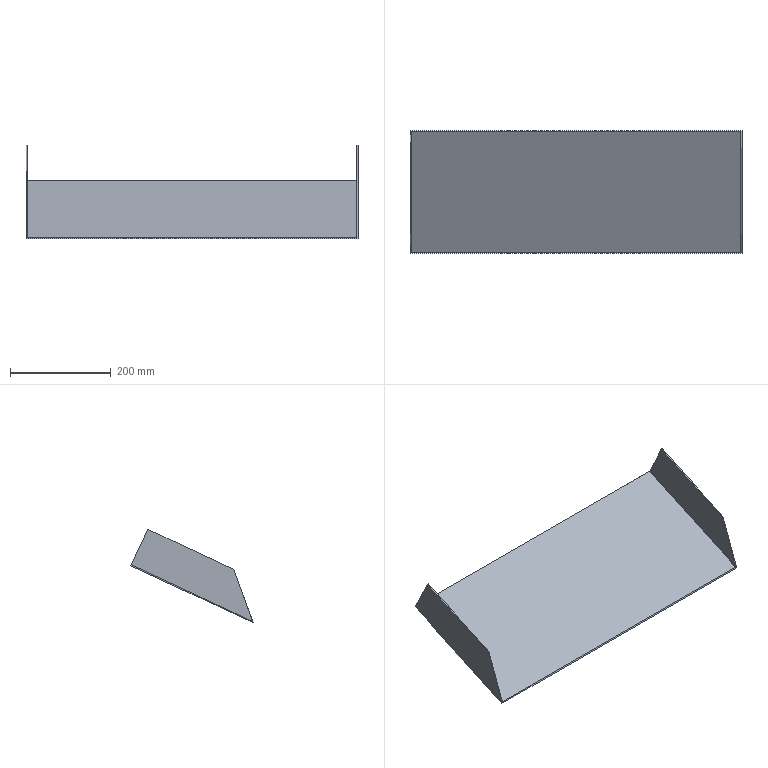Part | NX | features solid 2 | 1 solid | 10 faces | box 660 x 243.381 x 185.995 mm | volume 424148 mm3 | plane 10
STEP:
#1=CARTESIAN_POINT('',(708.,-733.725,-199.517));
#2=VERTEX_POINT('',#1);
#3=CARTESIAN_POINT('',(52.,-733.725,-199.517));
#4=VERTEX_POINT('',#3);
#5=CARTESIAN_POINT('',(1200.,-733.725,-199.517));
#6=DIRECTION('',(-1.,0.,0.));
#7=VECTOR('',#6,1000.);
#8=LINE('',#5,#7);
#9=EDGE_CURVE('',#2,#4,#8,.T.);
#10=ORIENTED_EDGE('',*,*,#9,.F.);
#11=CARTESIAN_POINT('',(708.,-766.69,-128.825));
#12=VERTEX_POINT('',#11);
#13=CARTESIAN_POINT('',(708.,-754.011,-156.015));
#14=DIRECTION('',(0.,-0.4226,0.9063));
#15=VECTOR('',#14,1000.);
#16=LINE('',#13,#15);
#17=EDGE_CURVE('',#2,#12,#16,.T.);
#18=ORIENTED_EDGE('',*,*,#17,.T.);
#19=CARTESIAN_POINT('',(710.,-766.69,-128.825));
#20=VERTEX_POINT('',#19);
#21=CARTESIAN_POINT('',(440.,-766.69,-128.825));
#22=DIRECTION('',(-1.,0.,0.));
#23=VECTOR('',#22,1000.);
#24=LINE('',#21,#23);
#25=EDGE_CURVE('',#20,#12,#24,.T.);
#26=ORIENTED_EDGE('',*,*,#25,.F.);
#27=CARTESIAN_POINT('',(710.,-732.88,-201.33));
#28=VERTEX_POINT('',#27);
#29=CARTESIAN_POINT('',(710.,-754.011,-156.015));
#30=DIRECTION('',(0.,-0.4226,0.9063));
#31=VECTOR('',#30,1000.);
#32=LINE('',#29,#31);
#33=EDGE_CURVE('',#28,#20,#32,.T.);
#34=ORIENTED_EDGE('',*,*,#33,.F.);
#35=CARTESIAN_POINT('',(50.,-732.88,-201.33));
#36=VERTEX_POINT('',#35);
#37=CARTESIAN_POINT('',(1200.,-732.88,-201.33));
#38=DIRECTION('',(-1.,0.,0.));
#39=VECTOR('',#38,1000.);
#40=LINE('',#37,#39);
#41=EDGE_CURVE('',#28,#36,#40,.T.);
#42=ORIENTED_EDGE('',*,*,#41,.T.);
#43=CARTESIAN_POINT('',(50.,-766.69,-128.825));
#44=VERTEX_POINT('',#43);
#45=CARTESIAN_POINT('',(50.,-754.011,-156.015));
#46=DIRECTION('',(0.,-0.4226,0.9063));
#47=VECTOR('',#46,1000.);
#48=LINE('',#45,#47);
#49=EDGE_CURVE('',#36,#44,#48,.T.);
#50=ORIENTED_EDGE('',*,*,#49,.T.);
#51=CARTESIAN_POINT('',(52.,-766.69,-128.825));
#52=VERTEX_POINT('',#51);
#53=CARTESIAN_POINT('',(320.,-766.69,-128.825));
#54=DIRECTION('',(1.,0.,0.));
#55=VECTOR('',#54,1000.);
#56=LINE('',#53,#55);
#57=EDGE_CURVE('',#44,#52,#56,.T.);
#58=ORIENTED_EDGE('',*,*,#57,.T.);
#59=CARTESIAN_POINT('',(52.,-754.011,-156.015));
#60=DIRECTION('',(0.,-0.4226,0.9063));
#61=VECTOR('',#60,1000.);
#62=LINE('',#59,#61);
#63=EDGE_CURVE('',#4,#52,#62,.T.);
#64=ORIENTED_EDGE('',*,*,#63,.F.);
#65=EDGE_LOOP('',(#10,#18,#26,#34,#42,#50,#58,#64));
#66=FACE_BOUND('',#65,.T.);
#67=CARTESIAN_POINT('',(1160.,-733.725,-199.517));
#68=DIRECTION('',(0.,0.9063,0.4226));
#69=DIRECTION('',(0.,-0.4226,0.9063));
#70=AXIS2_PLACEMENT_3D('',#67,#68,#69);
#71=PLANE('',#70);
#72=ADVANCED_FACE('',(#66),#71,.T.);
#73=ORIENTED_EDGE('',*,*,#41,.F.);
#74=CARTESIAN_POINT('',(710.,-976.262,-314.821));
#75=VERTEX_POINT('',#74);
#76=CARTESIAN_POINT('',(710.,235.,250.));
#77=DIRECTION('',(0.,-0.9063,-0.4226));
#78=VECTOR('',#77,1000.);
#79=LINE('',#76,#78);
#80=EDGE_CURVE('',#28,#75,#79,.T.);
#81=ORIENTED_EDGE('',*,*,#80,.T.);
#82=CARTESIAN_POINT('',(50.,-976.262,-314.821));
#83=VERTEX_POINT('',#82);
#84=CARTESIAN_POINT('',(1200.,-976.262,-314.821));
#85=DIRECTION('',(-1.,0.,0.));
#86=VECTOR('',#85,1000.);
#87=LINE('',#84,#86);
#88=EDGE_CURVE('',#75,#83,#87,.T.);
#89=ORIENTED_EDGE('',*,*,#88,.T.);
#90=CARTESIAN_POINT('',(50.,235.,250.));
#91=DIRECTION('',(0.,-0.9063,-0.4226));
#92=VECTOR('',#91,1000.);
#93=LINE('',#90,#92);
#94=EDGE_CURVE('',#36,#83,#93,.T.);
#95=ORIENTED_EDGE('',*,*,#94,.F.);
#96=EDGE_LOOP('',(#73,#81,#89,#95));
#97=FACE_BOUND('',#96,.T.);
#98=CARTESIAN_POINT('',(1200.,235.,250.));
#99=DIRECTION('',(0.,0.4226,-0.9063));
#100=DIRECTION('',(0.,-0.9063,-0.4226));
#101=AXIS2_PLACEMENT_3D('',#98,#99,#100);
#102=PLANE('',#101);
#103=ADVANCED_FACE('',(#97),#102,.T.);
#104=ORIENTED_EDGE('',*,*,#9,.T.);
#105=CARTESIAN_POINT('',(52.,-975.294,-312.163));
#106=VERTEX_POINT('',#105);
#107=CARTESIAN_POINT('',(52.,234.155,251.813));
#108=DIRECTION('',(0.,-0.9063,-0.4226));
#109=VECTOR('',#108,1000.);
#110=LINE('',#107,#109);
#111=EDGE_CURVE('',#4,#106,#110,.T.);
#112=ORIENTED_EDGE('',*,*,#111,.T.);
#113=CARTESIAN_POINT('',(708.,-975.294,-312.163));
#114=VERTEX_POINT('',#113);
#115=CARTESIAN_POINT('',(1200.,-975.294,-312.163));
#116=DIRECTION('',(1.,0.,0.));
#117=VECTOR('',#116,1000.);
#118=LINE('',#115,#117);
#119=EDGE_CURVE('',#114,#106,#118,.F.);
#120=ORIENTED_EDGE('',*,*,#119,.F.);
#121=CARTESIAN_POINT('',(708.,234.155,251.813));
#122=DIRECTION('',(0.,-0.9063,-0.4226));
#123=VECTOR('',#122,1000.);
#124=LINE('',#121,#123);
#125=EDGE_CURVE('',#2,#114,#124,.T.);
#126=ORIENTED_EDGE('',*,*,#125,.F.);
#127=EDGE_LOOP('',(#104,#112,#120,#126));
#128=FACE_BOUND('',#127,.T.);
#129=CARTESIAN_POINT('',(1200.,234.155,251.813));
#130=DIRECTION('',(0.,0.4226,-0.9063));
#131=DIRECTION('',(0.,-0.9063,-0.4226));
#132=AXIS2_PLACEMENT_3D('',#129,#130,#131);
#133=PLANE('',#132);
#134=ADVANCED_FACE('',(#128),#133,.F.);
#135=ORIENTED_EDGE('',*,*,#88,.F.);
#136=CARTESIAN_POINT('',(710.,-937.566,-208.506));
#137=VERTEX_POINT('',#136);
#138=CARTESIAN_POINT('',(710.,-937.566,-208.506));
#139=DIRECTION('',(0.,-0.342,-0.9397));
#140=VECTOR('',#139,1000.);
#141=LINE('',#138,#140);
#142=EDGE_CURVE('',#75,#137,#141,.F.);
#143=ORIENTED_EDGE('',*,*,#142,.T.);
#144=CARTESIAN_POINT('',(708.,-937.566,-208.506));
#145=VERTEX_POINT('',#144);
#146=CARTESIAN_POINT('',(440.,-937.566,-208.506));
#147=DIRECTION('',(1.,0.,0.));
#148=VECTOR('',#147,1000.);
#149=LINE('',#146,#148);
#150=EDGE_CURVE('',#137,#145,#149,.F.);
#151=ORIENTED_EDGE('',*,*,#150,.T.);
#152=CARTESIAN_POINT('',(708.,-640.949,606.444));
#153=DIRECTION('',(0.,0.342,0.9397));
#154=VECTOR('',#153,1000.);
#155=LINE('',#152,#154);
#156=EDGE_CURVE('',#145,#114,#155,.F.);
#157=ORIENTED_EDGE('',*,*,#156,.T.);
#158=ORIENTED_EDGE('',*,*,#119,.T.);
#159=CARTESIAN_POINT('',(52.,-937.566,-208.506));
#160=VERTEX_POINT('',#159);
#161=CARTESIAN_POINT('',(52.,-640.949,606.444));
#162=DIRECTION('',(0.,0.342,0.9397));
#163=VECTOR('',#162,1000.);
#164=LINE('',#161,#163);
#165=EDGE_CURVE('',#160,#106,#164,.F.);
#166=ORIENTED_EDGE('',*,*,#165,.F.);
#167=CARTESIAN_POINT('',(50.,-937.566,-208.506));
#168=VERTEX_POINT('',#167);
#169=CARTESIAN_POINT('',(320.,-937.566,-208.506));
#170=DIRECTION('',(-1.,0.,0.));
#171=VECTOR('',#170,1000.);
#172=LINE('',#169,#171);
#173=EDGE_CURVE('',#168,#160,#172,.F.);
#174=ORIENTED_EDGE('',*,*,#173,.F.);
#175=CARTESIAN_POINT('',(50.,-937.566,-208.506));
#176=DIRECTION('',(0.,-0.342,-0.9397));
#177=VECTOR('',#176,1000.);
#178=LINE('',#175,#177);
#179=EDGE_CURVE('',#83,#168,#178,.F.);
#180=ORIENTED_EDGE('',*,*,#179,.F.);
#181=EDGE_LOOP('',(#135,#143,#151,#157,#158,#166,#174,#180));
#182=FACE_BOUND('',#181,.T.);
#183=CARTESIAN_POINT('',(1200.,-937.566,-208.506));
#184=DIRECTION('',(0.,0.9397,-0.342));
#185=DIRECTION('',(0.,0.342,0.9397));
#186=AXIS2_PLACEMENT_3D('',#183,#184,#185);
#187=PLANE('',#186);
#188=ADVANCED_FACE('',(#182),#187,.F.);
#189=ORIENTED_EDGE('',*,*,#57,.F.);
#190=CARTESIAN_POINT('',(50.,201.191,322.505));
#191=DIRECTION('',(0.,-0.9063,-0.4226));
#192=VECTOR('',#191,1000.);
#193=LINE('',#190,#192);
#194=EDGE_CURVE('',#44,#168,#193,.T.);
#195=ORIENTED_EDGE('',*,*,#194,.T.);
#196=ORIENTED_EDGE('',*,*,#173,.T.);
#197=CARTESIAN_POINT('',(52.,201.191,322.505));
#198=DIRECTION('',(0.,-0.9063,-0.4226));
#199=VECTOR('',#198,1000.);
#200=LINE('',#197,#199);
#201=EDGE_CURVE('',#52,#160,#200,.T.);
#202=ORIENTED_EDGE('',*,*,#201,.F.);
#203=EDGE_LOOP('',(#189,#195,#196,#202));
#204=FACE_BOUND('',#203,.T.);
#205=CARTESIAN_POINT('',(320.,201.191,322.505));
#206=DIRECTION('',(0.,0.4226,-0.9063));
#207=DIRECTION('',(0.,-0.9063,-0.4226));
#208=AXIS2_PLACEMENT_3D('',#205,#206,#207);
#209=PLANE('',#208);
#210=ADVANCED_FACE('',(#204),#209,.F.);
#211=ORIENTED_EDGE('',*,*,#49,.F.);
#212=ORIENTED_EDGE('',*,*,#94,.T.);
#213=ORIENTED_EDGE('',*,*,#179,.T.);
#214=ORIENTED_EDGE('',*,*,#194,.F.);
#215=EDGE_LOOP('',(#211,#212,#213,#214));
#216=FACE_BOUND('',#215,.T.);
#217=CARTESIAN_POINT('',(50.,213.869,295.315));
#218=DIRECTION('',(1.,0.,0.));
#219=DIRECTION('',(0.,0.,-1.));
#220=AXIS2_PLACEMENT_3D('',#217,#218,#219);
#221=PLANE('',#220);
#222=ADVANCED_FACE('',(#216),#221,.F.);
#223=ORIENTED_EDGE('',*,*,#111,.F.);
#224=ORIENTED_EDGE('',*,*,#63,.T.);
#225=ORIENTED_EDGE('',*,*,#201,.T.);
#226=ORIENTED_EDGE('',*,*,#165,.T.);
#227=EDGE_LOOP('',(#223,#224,#225,#226));
#228=FACE_BOUND('',#227,.T.);
#229=CARTESIAN_POINT('',(52.,213.869,295.315));
#230=DIRECTION('',(1.,0.,0.));
#231=DIRECTION('',(0.,0.,-1.));
#232=AXIS2_PLACEMENT_3D('',#229,#230,#231);
#233=PLANE('',#232);
#234=ADVANCED_FACE('',(#228),#233,.T.);
#235=ORIENTED_EDGE('',*,*,#25,.T.);
#236=CARTESIAN_POINT('',(708.,201.191,322.505));
#237=DIRECTION('',(0.,-0.9063,-0.4226));
#238=VECTOR('',#237,1000.);
#239=LINE('',#236,#238);
#240=EDGE_CURVE('',#12,#145,#239,.T.);
#241=ORIENTED_EDGE('',*,*,#240,.T.);
#242=ORIENTED_EDGE('',*,*,#150,.F.);
#243=CARTESIAN_POINT('',(710.,201.191,322.505));
#244=DIRECTION('',(0.,-0.9063,-0.4226));
#245=VECTOR('',#244,1000.);
#246=LINE('',#243,#245);
#247=EDGE_CURVE('',#20,#137,#246,.T.);
#248=ORIENTED_EDGE('',*,*,#247,.F.);
#249=EDGE_LOOP('',(#235,#241,#242,#248));
#250=FACE_BOUND('',#249,.T.);
#251=CARTESIAN_POINT('',(440.,201.191,322.505));
#252=DIRECTION('',(0.,0.4226,-0.9063));
#253=DIRECTION('',(0.,-0.9063,-0.4226));
#254=AXIS2_PLACEMENT_3D('',#251,#252,#253);
#255=PLANE('',#254);
#256=ADVANCED_FACE('',(#250),#255,.F.);
#257=ORIENTED_EDGE('',*,*,#33,.T.);
#258=ORIENTED_EDGE('',*,*,#247,.T.);
#259=ORIENTED_EDGE('',*,*,#142,.F.);
#260=ORIENTED_EDGE('',*,*,#80,.F.);
#261=EDGE_LOOP('',(#257,#258,#259,#260));
#262=FACE_BOUND('',#261,.T.);
#263=CARTESIAN_POINT('',(710.,213.869,295.315));
#264=DIRECTION('',(-1.,0.,0.));
#265=DIRECTION('',(0.,0.,-1.));
#266=AXIS2_PLACEMENT_3D('',#263,#264,#265);
#267=PLANE('',#266);
#268=ADVANCED_FACE('',(#262),#267,.F.);
#269=ORIENTED_EDGE('',*,*,#125,.T.);
#270=ORIENTED_EDGE('',*,*,#156,.F.);
#271=ORIENTED_EDGE('',*,*,#240,.F.);
#272=ORIENTED_EDGE('',*,*,#17,.F.);
#273=EDGE_LOOP('',(#269,#270,#271,#272));
#274=FACE_BOUND('',#273,.T.);
#275=CARTESIAN_POINT('',(708.,213.869,295.315));
#276=DIRECTION('',(-1.,0.,0.));
#277=DIRECTION('',(0.,0.,-1.));
#278=AXIS2_PLACEMENT_3D('',#275,#276,#277);
#279=PLANE('',#278);
#280=ADVANCED_FACE('',(#274),#279,.T.);
#281=CLOSED_SHELL('',(#72,#103,#134,#188,#210,#222,#234,#256,#268,#280));
#282=MANIFOLD_SOLID_BREP('',#281);
#283=(LENGTH_UNIT()NAMED_UNIT(*)SI_UNIT(.MILLI.,.METRE.));
#284=UNCERTAINTY_MEASURE_WITH_UNIT(LENGTH_MEASURE(0.00001),#283,'','');
#285=(NAMED_UNIT(*)PLANE_ANGLE_UNIT()SI_UNIT($,.RADIAN.));
#286=(NAMED_UNIT(*)SI_UNIT($,.STERADIAN.)SOLID_ANGLE_UNIT());
#287=(GEOMETRIC_REPRESENTATION_CONTEXT(3)GLOBAL_UNCERTAINTY_ASSIGNED_CONTEXT((#284))GLOBAL_UNIT_ASSIGNED_CONTEXT((#283,#285,#286))REPRESENTATION_CONTEXT('',''));
#288=ADVANCED_BREP_SHAPE_REPRESENTATION('',(#282),#287);